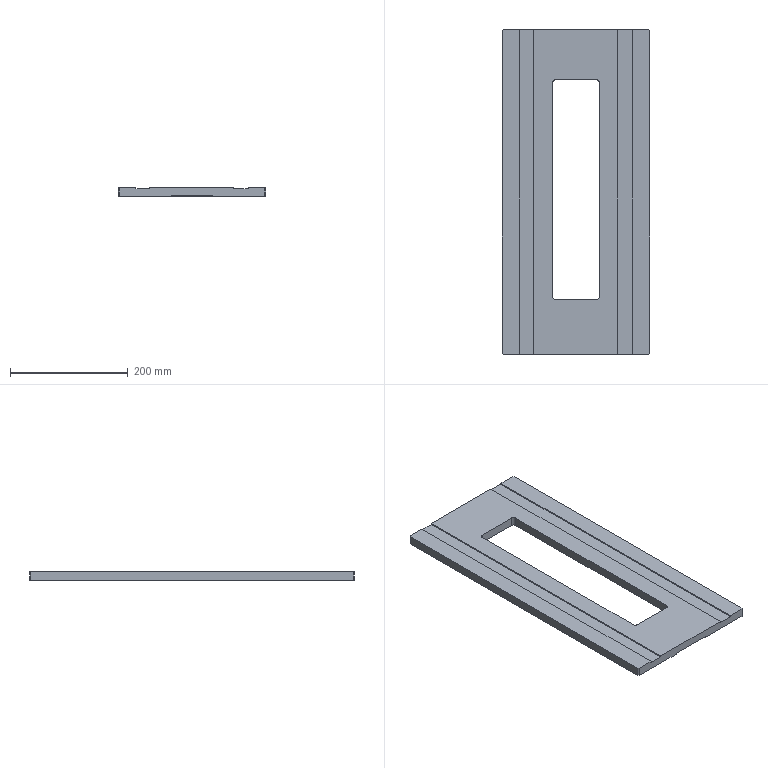Part | STEP file | 001-003-Storage mechanism vertical plate | 1 solid | 44 faces | box 250 x 550 x 15 mm | volume 1550347 mm3 | plane 31 | cylinder 13 | commonest cylinder face diameters 6 x9 10 x4